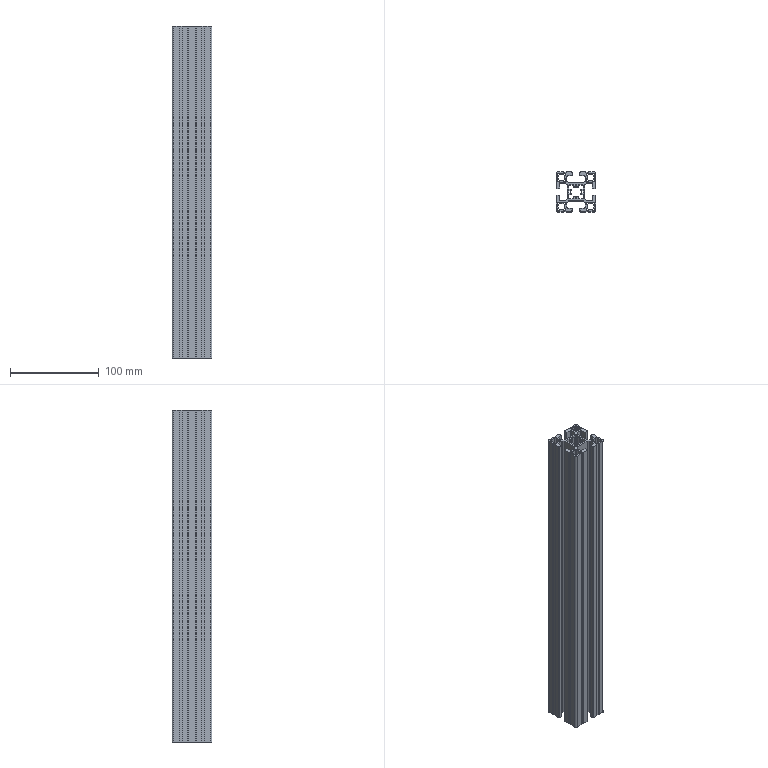Part | STEP file | 4545 profile NG mount 3 | 1 solid | 262 faces | box 45 x 45 x 375 mm | volume 260193 mm3 | plane 186 | cylinder 76 | commonest cylinder face diameters 2 x44 8 x20 12 x8 4 x4